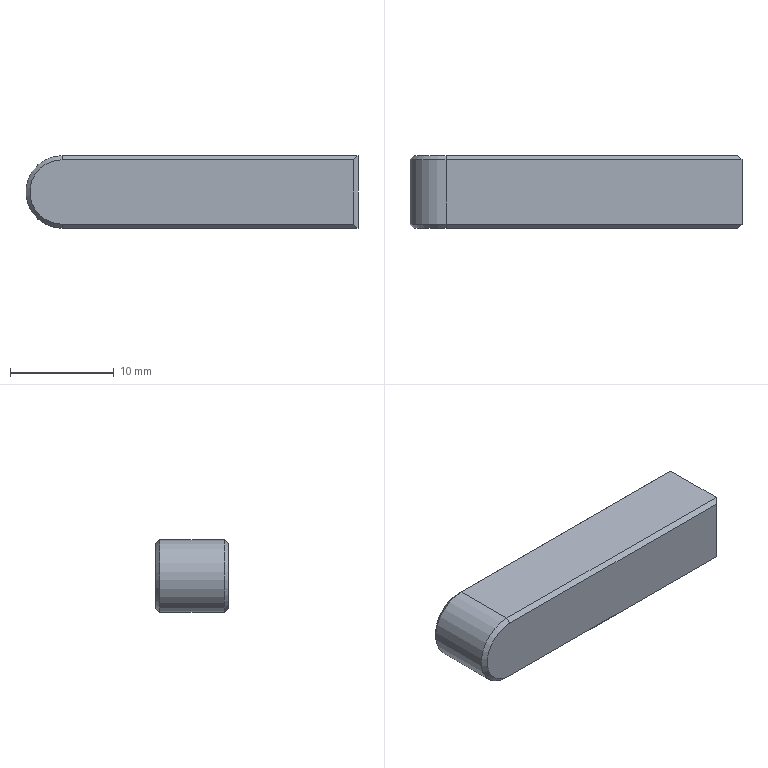Part | SolidWorks | features Chamfer 1, Extrusion 1 | 1 solid | 14 faces | box 32 x 7 x 7 mm | volume 1519 mm3 | plane 11 | cone 2 | cylinder 1 | commonest cylinder face diameters 7 x1
STEP:
#1=CARTESIAN_POINT('',(3.5,6.6,7.));
#2=VERTEX_POINT('',#1);
#3=CARTESIAN_POINT('',(3.5,0.4,7.));
#4=VERTEX_POINT('',#3);
#5=CARTESIAN_POINT('',(3.5,7.,7.));
#6=DIRECTION('',(0.,-1.,0.));
#7=VECTOR('',#6,1000.);
#8=LINE('',#5,#7);
#9=EDGE_CURVE('',#2,#4,#8,.T.);
#10=ORIENTED_EDGE('',*,*,#9,.F.);
#11=CARTESIAN_POINT('',(3.5,6.6,0.));
#12=VERTEX_POINT('',#11);
#13=CARTESIAN_POINT('',(3.5,6.6,3.5));
#14=DIRECTION('',(0.,-1.,0.));
#15=DIRECTION('',(0.,0.,1.));
#16=AXIS2_PLACEMENT_3D('',#13,#14,#15);
#17=CIRCLE('',#16,3.5);
#18=EDGE_CURVE('',#2,#12,#17,.T.);
#19=ORIENTED_EDGE('',*,*,#18,.T.);
#20=CARTESIAN_POINT('',(3.5,0.4,0.));
#21=VERTEX_POINT('',#20);
#22=CARTESIAN_POINT('',(3.5,7.,0.));
#23=DIRECTION('',(0.,-1.,0.));
#24=VECTOR('',#23,1000.);
#25=LINE('',#22,#24);
#26=EDGE_CURVE('',#12,#21,#25,.T.);
#27=ORIENTED_EDGE('',*,*,#26,.T.);
#28=CARTESIAN_POINT('',(3.5,0.4,3.5));
#29=DIRECTION('',(0.,1.,0.));
#30=DIRECTION('',(0.,0.,1.));
#31=AXIS2_PLACEMENT_3D('',#28,#29,#30);
#32=CIRCLE('',#31,3.5);
#33=EDGE_CURVE('',#21,#4,#32,.T.);
#34=ORIENTED_EDGE('',*,*,#33,.T.);
#35=EDGE_LOOP('',(#10,#19,#27,#34));
#36=FACE_OUTER_BOUND('',#35,.T.);
#37=CARTESIAN_POINT('',(3.5,7.,3.5));
#38=DIRECTION('',(0.,-1.,0.));
#39=DIRECTION('',(0.,0.,-1.));
#40=AXIS2_PLACEMENT_3D('',#37,#38,#39);
#41=CYLINDRICAL_SURFACE('',#40,3.5);
#42=ADVANCED_FACE('',(#36),#41,.T.);
#43=CARTESIAN_POINT('',(32.,6.6,7.));
#44=VERTEX_POINT('',#43);
#45=CARTESIAN_POINT('',(32.,0.4,7.));
#46=VERTEX_POINT('',#45);
#47=CARTESIAN_POINT('',(32.,7.,7.));
#48=DIRECTION('',(0.,-1.,0.));
#49=VECTOR('',#48,1000.);
#50=LINE('',#47,#49);
#51=EDGE_CURVE('',#44,#46,#50,.T.);
#52=ORIENTED_EDGE('',*,*,#51,.F.);
#53=CARTESIAN_POINT('',(3.5,6.6,7.));
#54=DIRECTION('',(-1.,0.,0.));
#55=VECTOR('',#54,1000.);
#56=LINE('',#53,#55);
#57=EDGE_CURVE('',#44,#2,#56,.T.);
#58=ORIENTED_EDGE('',*,*,#57,.T.);
#59=ORIENTED_EDGE('',*,*,#9,.T.);
#60=CARTESIAN_POINT('',(3.5,0.4,7.));
#61=DIRECTION('',(1.,0.,0.));
#62=VECTOR('',#61,1000.);
#63=LINE('',#60,#62);
#64=EDGE_CURVE('',#4,#46,#63,.T.);
#65=ORIENTED_EDGE('',*,*,#64,.T.);
#66=EDGE_LOOP('',(#52,#58,#59,#65));
#67=FACE_OUTER_BOUND('',#66,.T.);
#68=CARTESIAN_POINT('',(3.5,7.,7.));
#69=DIRECTION('',(0.,0.,-1.));
#70=DIRECTION('',(-1.,0.,0.));
#71=AXIS2_PLACEMENT_3D('',#68,#69,#70);
#72=PLANE('',#71);
#73=ADVANCED_FACE('',(#67),#72,.F.);
#74=CARTESIAN_POINT('',(32.,6.6,0.));
#75=VERTEX_POINT('',#74);
#76=CARTESIAN_POINT('',(32.,0.4,0.));
#77=VERTEX_POINT('',#76);
#78=CARTESIAN_POINT('',(32.,7.,0.));
#79=DIRECTION('',(0.,-1.,0.));
#80=VECTOR('',#79,1000.);
#81=LINE('',#78,#80);
#82=EDGE_CURVE('',#75,#77,#81,.T.);
#83=ORIENTED_EDGE('',*,*,#82,.F.);
#84=CARTESIAN_POINT('',(32.,6.6,0.));
#85=DIRECTION('',(0.,0.,1.));
#86=VECTOR('',#85,1000.);
#87=LINE('',#84,#86);
#88=EDGE_CURVE('',#75,#44,#87,.T.);
#89=ORIENTED_EDGE('',*,*,#88,.T.);
#90=ORIENTED_EDGE('',*,*,#51,.T.);
#91=CARTESIAN_POINT('',(32.,0.4,0.));
#92=DIRECTION('',(0.,0.,-1.));
#93=VECTOR('',#92,1000.);
#94=LINE('',#91,#93);
#95=EDGE_CURVE('',#46,#77,#94,.T.);
#96=ORIENTED_EDGE('',*,*,#95,.T.);
#97=EDGE_LOOP('',(#83,#89,#90,#96));
#98=FACE_OUTER_BOUND('',#97,.T.);
#99=CARTESIAN_POINT('',(32.,7.,0.));
#100=DIRECTION('',(1.,0.,0.));
#101=DIRECTION('',(0.,0.,-1.));
#102=AXIS2_PLACEMENT_3D('',#99,#100,#101);
#103=PLANE('',#102);
#104=ADVANCED_FACE('',(#98),#103,.T.);
#105=ORIENTED_EDGE('',*,*,#26,.F.);
#106=CARTESIAN_POINT('',(3.5,6.6,0.));
#107=DIRECTION('',(1.,0.,0.));
#108=VECTOR('',#107,1000.);
#109=LINE('',#106,#108);
#110=EDGE_CURVE('',#12,#75,#109,.T.);
#111=ORIENTED_EDGE('',*,*,#110,.T.);
#112=ORIENTED_EDGE('',*,*,#82,.T.);
#113=CARTESIAN_POINT('',(3.5,0.4,0.));
#114=DIRECTION('',(-1.,0.,0.));
#115=VECTOR('',#114,1000.);
#116=LINE('',#113,#115);
#117=EDGE_CURVE('',#77,#21,#116,.T.);
#118=ORIENTED_EDGE('',*,*,#117,.T.);
#119=EDGE_LOOP('',(#105,#111,#112,#118));
#120=FACE_OUTER_BOUND('',#119,.T.);
#121=CARTESIAN_POINT('',(3.5,7.,0.));
#122=DIRECTION('',(0.,0.,-1.));
#123=DIRECTION('',(-1.,0.,0.));
#124=AXIS2_PLACEMENT_3D('',#121,#122,#123);
#125=PLANE('',#124);
#126=ADVANCED_FACE('',(#120),#125,.T.);
#127=CARTESIAN_POINT('',(3.5,7.,6.6));
#128=VERTEX_POINT('',#127);
#129=CARTESIAN_POINT('',(31.6,7.,6.6));
#130=VERTEX_POINT('',#129);
#131=CARTESIAN_POINT('',(32.,7.,6.6));
#132=DIRECTION('',(1.,0.,0.));
#133=VECTOR('',#132,1000.);
#134=LINE('',#131,#133);
#135=EDGE_CURVE('',#128,#130,#134,.T.);
#136=ORIENTED_EDGE('',*,*,#135,.T.);
#137=CARTESIAN_POINT('',(31.6,7.,0.4));
#138=VERTEX_POINT('',#137);
#139=CARTESIAN_POINT('',(31.6,7.,3.5));
#140=DIRECTION('',(0.,0.,-1.));
#141=VECTOR('',#140,1000.);
#142=LINE('',#139,#141);
#143=EDGE_CURVE('',#130,#138,#142,.T.);
#144=ORIENTED_EDGE('',*,*,#143,.T.);
#145=CARTESIAN_POINT('',(3.5,7.,0.4));
#146=VERTEX_POINT('',#145);
#147=CARTESIAN_POINT('',(3.5,7.,0.4));
#148=DIRECTION('',(-1.,0.,0.));
#149=VECTOR('',#148,1000.);
#150=LINE('',#147,#149);
#151=EDGE_CURVE('',#138,#146,#150,.T.);
#152=ORIENTED_EDGE('',*,*,#151,.T.);
#153=CARTESIAN_POINT('',(3.5,7.,3.5));
#154=DIRECTION('',(0.,1.,0.));
#155=DIRECTION('',(0.,0.,1.));
#156=AXIS2_PLACEMENT_3D('',#153,#154,#155);
#157=CIRCLE('',#156,3.1);
#158=EDGE_CURVE('',#146,#128,#157,.T.);
#159=ORIENTED_EDGE('',*,*,#158,.T.);
#160=EDGE_LOOP('',(#136,#144,#152,#159));
#161=FACE_OUTER_BOUND('',#160,.T.);
#162=CARTESIAN_POINT('',(3.5,7.,3.5));
#163=DIRECTION('',(0.,1.,0.));
#164=DIRECTION('',(0.,0.,1.));
#165=AXIS2_PLACEMENT_3D('',#162,#163,#164);
#166=PLANE('',#165);
#167=ADVANCED_FACE('',(#161),#166,.T.);
#168=CARTESIAN_POINT('',(3.5,0.,0.4));
#169=VERTEX_POINT('',#168);
#170=CARTESIAN_POINT('',(31.6,0.,0.4));
#171=VERTEX_POINT('',#170);
#172=CARTESIAN_POINT('',(32.,0.,0.4));
#173=DIRECTION('',(1.,0.,0.));
#174=VECTOR('',#173,1000.);
#175=LINE('',#172,#174);
#176=EDGE_CURVE('',#169,#171,#175,.T.);
#177=ORIENTED_EDGE('',*,*,#176,.T.);
#178=CARTESIAN_POINT('',(31.6,0.,6.6));
#179=VERTEX_POINT('',#178);
#180=CARTESIAN_POINT('',(31.6,0.,7.));
#181=DIRECTION('',(0.,0.,1.));
#182=VECTOR('',#181,1000.);
#183=LINE('',#180,#182);
#184=EDGE_CURVE('',#171,#179,#183,.T.);
#185=ORIENTED_EDGE('',*,*,#184,.T.);
#186=CARTESIAN_POINT('',(3.5,0.,6.6));
#187=VERTEX_POINT('',#186);
#188=CARTESIAN_POINT('',(3.5,0.,6.6));
#189=DIRECTION('',(-1.,0.,0.));
#190=VECTOR('',#189,1000.);
#191=LINE('',#188,#190);
#192=EDGE_CURVE('',#179,#187,#191,.T.);
#193=ORIENTED_EDGE('',*,*,#192,.T.);
#194=CARTESIAN_POINT('',(3.5,0.,3.5));
#195=DIRECTION('',(0.,-1.,0.));
#196=DIRECTION('',(0.,0.,1.));
#197=AXIS2_PLACEMENT_3D('',#194,#195,#196);
#198=CIRCLE('',#197,3.1);
#199=EDGE_CURVE('',#187,#169,#198,.T.);
#200=ORIENTED_EDGE('',*,*,#199,.T.);
#201=EDGE_LOOP('',(#177,#185,#193,#200));
#202=FACE_OUTER_BOUND('',#201,.T.);
#203=CARTESIAN_POINT('',(3.5,0.,3.5));
#204=DIRECTION('',(0.,1.,0.));
#205=DIRECTION('',(0.,0.,1.));
#206=AXIS2_PLACEMENT_3D('',#203,#204,#205);
#207=PLANE('',#206);
#208=ADVANCED_FACE('',(#202),#207,.F.);
#209=CARTESIAN_POINT('',(3.5,7.,6.6));
#210=DIRECTION('',(0.,-0.7071,0.7071));
#211=VECTOR('',#210,1000.);
#212=LINE('',#209,#211);
#213=EDGE_CURVE('',#128,#2,#212,.T.);
#214=ORIENTED_EDGE('',*,*,#213,.F.);
#215=ORIENTED_EDGE('',*,*,#158,.F.);
#216=CARTESIAN_POINT('',(3.5,6.6,0.));
#217=DIRECTION('',(0.,0.7071,0.7071));
#218=VECTOR('',#217,1000.);
#219=LINE('',#216,#218);
#220=EDGE_CURVE('',#12,#146,#219,.T.);
#221=ORIENTED_EDGE('',*,*,#220,.F.);
#222=ORIENTED_EDGE('',*,*,#18,.F.);
#223=EDGE_LOOP('',(#214,#215,#221,#222));
#224=FACE_OUTER_BOUND('',#223,.T.);
#225=CARTESIAN_POINT('',(3.5,7.,3.5));
#226=DIRECTION('',(0.,-1.,0.));
#227=DIRECTION('',(0.,0.,-1.));
#228=AXIS2_PLACEMENT_3D('',#225,#226,#227);
#229=CONICAL_SURFACE('',#228,3.1,0.7854);
#230=ADVANCED_FACE('',(#224),#229,.T.);
#231=ORIENTED_EDGE('',*,*,#220,.T.);
#232=ORIENTED_EDGE('',*,*,#151,.F.);
#233=CARTESIAN_POINT('',(22.5,16.1,9.5));
#234=DIRECTION('',(-0.5774,0.5774,0.5774));
#235=VECTOR('',#234,1000.);
#236=LINE('',#233,#235);
#237=EDGE_CURVE('',#75,#138,#236,.T.);
#238=ORIENTED_EDGE('',*,*,#237,.F.);
#239=ORIENTED_EDGE('',*,*,#110,.F.);
#240=EDGE_LOOP('',(#231,#232,#238,#239));
#241=FACE_OUTER_BOUND('',#240,.T.);
#242=CARTESIAN_POINT('',(3.5,6.6,0.));
#243=DIRECTION('',(0.,-0.7071,0.7071));
#244=DIRECTION('',(1.,0.,0.));
#245=AXIS2_PLACEMENT_3D('',#242,#243,#244);
#246=PLANE('',#245);
#247=ADVANCED_FACE('',(#241),#246,.F.);
#248=ORIENTED_EDGE('',*,*,#213,.T.);
#249=ORIENTED_EDGE('',*,*,#57,.F.);
#250=CARTESIAN_POINT('',(22.233,16.367,-2.767));
#251=DIRECTION('',(0.5774,-0.5774,0.5774));
#252=VECTOR('',#251,1000.);
#253=LINE('',#250,#252);
#254=EDGE_CURVE('',#130,#44,#253,.T.);
#255=ORIENTED_EDGE('',*,*,#254,.F.);
#256=ORIENTED_EDGE('',*,*,#135,.F.);
#257=EDGE_LOOP('',(#248,#249,#255,#256));
#258=FACE_OUTER_BOUND('',#257,.T.);
#259=CARTESIAN_POINT('',(3.5,7.,6.6));
#260=DIRECTION('',(0.,0.7071,0.7071));
#261=DIRECTION('',(-1.,0.,0.));
#262=AXIS2_PLACEMENT_3D('',#259,#260,#261);
#263=PLANE('',#262);
#264=ADVANCED_FACE('',(#258),#263,.T.);
#265=ORIENTED_EDGE('',*,*,#237,.T.);
#266=ORIENTED_EDGE('',*,*,#143,.F.);
#267=ORIENTED_EDGE('',*,*,#254,.T.);
#268=ORIENTED_EDGE('',*,*,#88,.F.);
#269=EDGE_LOOP('',(#265,#266,#267,#268));
#270=FACE_OUTER_BOUND('',#269,.T.);
#271=CARTESIAN_POINT('',(32.,6.6,0.));
#272=DIRECTION('',(-0.7071,-0.7071,0.));
#273=DIRECTION('',(0.,0.,1.));
#274=AXIS2_PLACEMENT_3D('',#271,#272,#273);
#275=PLANE('',#274);
#276=ADVANCED_FACE('',(#270),#275,.F.);
#277=CARTESIAN_POINT('',(3.5,0.4,7.));
#278=DIRECTION('',(0.,-0.7071,-0.7071));
#279=VECTOR('',#278,1000.);
#280=LINE('',#277,#279);
#281=EDGE_CURVE('',#4,#187,#280,.T.);
#282=ORIENTED_EDGE('',*,*,#281,.F.);
#283=ORIENTED_EDGE('',*,*,#33,.F.);
#284=CARTESIAN_POINT('',(3.5,0.,0.4));
#285=DIRECTION('',(0.,0.7071,-0.7071));
#286=VECTOR('',#285,1000.);
#287=LINE('',#284,#286);
#288=EDGE_CURVE('',#169,#21,#287,.T.);
#289=ORIENTED_EDGE('',*,*,#288,.F.);
#290=ORIENTED_EDGE('',*,*,#199,.F.);
#291=EDGE_LOOP('',(#282,#283,#289,#290));
#292=FACE_OUTER_BOUND('',#291,.T.);
#293=CARTESIAN_POINT('',(3.5,0.4,3.5));
#294=DIRECTION('',(0.,1.,0.));
#295=DIRECTION('',(0.,0.,1.));
#296=AXIS2_PLACEMENT_3D('',#293,#294,#295);
#297=CONICAL_SURFACE('',#296,3.5,0.7854);
#298=ADVANCED_FACE('',(#292),#297,.T.);
#299=ORIENTED_EDGE('',*,*,#288,.T.);
#300=ORIENTED_EDGE('',*,*,#117,.F.);
#301=CARTESIAN_POINT('',(22.233,-9.367,9.767));
#302=DIRECTION('',(0.5774,0.5774,-0.5774));
#303=VECTOR('',#302,1000.);
#304=LINE('',#301,#303);
#305=EDGE_CURVE('',#171,#77,#304,.T.);
#306=ORIENTED_EDGE('',*,*,#305,.F.);
#307=ORIENTED_EDGE('',*,*,#176,.F.);
#308=EDGE_LOOP('',(#299,#300,#306,#307));
#309=FACE_OUTER_BOUND('',#308,.T.);
#310=CARTESIAN_POINT('',(3.5,0.,0.4));
#311=DIRECTION('',(0.,-0.7071,-0.7071));
#312=DIRECTION('',(-1.,0.,0.));
#313=AXIS2_PLACEMENT_3D('',#310,#311,#312);
#314=PLANE('',#313);
#315=ADVANCED_FACE('',(#309),#314,.T.);
#316=ORIENTED_EDGE('',*,*,#281,.T.);
#317=ORIENTED_EDGE('',*,*,#192,.F.);
#318=CARTESIAN_POINT('',(22.5,-9.1,-2.5));
#319=DIRECTION('',(-0.5774,-0.5774,-0.5774));
#320=VECTOR('',#319,1000.);
#321=LINE('',#318,#320);
#322=EDGE_CURVE('',#46,#179,#321,.T.);
#323=ORIENTED_EDGE('',*,*,#322,.F.);
#324=ORIENTED_EDGE('',*,*,#64,.F.);
#325=EDGE_LOOP('',(#316,#317,#323,#324));
#326=FACE_OUTER_BOUND('',#325,.T.);
#327=CARTESIAN_POINT('',(3.5,0.4,7.));
#328=DIRECTION('',(0.,0.7071,-0.7071));
#329=DIRECTION('',(1.,0.,0.));
#330=AXIS2_PLACEMENT_3D('',#327,#328,#329);
#331=PLANE('',#330);
#332=ADVANCED_FACE('',(#326),#331,.F.);
#333=ORIENTED_EDGE('',*,*,#305,.T.);
#334=ORIENTED_EDGE('',*,*,#95,.F.);
#335=ORIENTED_EDGE('',*,*,#322,.T.);
#336=ORIENTED_EDGE('',*,*,#184,.F.);
#337=EDGE_LOOP('',(#333,#334,#335,#336));
#338=FACE_OUTER_BOUND('',#337,.T.);
#339=CARTESIAN_POINT('',(31.6,0.,3.5));
#340=DIRECTION('',(0.7071,-0.7071,0.));
#341=DIRECTION('',(0.,0.,-1.));
#342=AXIS2_PLACEMENT_3D('',#339,#340,#341);
#343=PLANE('',#342);
#344=ADVANCED_FACE('',(#338),#343,.T.);
#345=CLOSED_SHELL('',(#42,#73,#104,#126,#167,#208,#230,#247,#264,#276,#298,#315,#332,#344));
#346=MANIFOLD_SOLID_BREP('',#345);
#347=CARTESIAN_POINT('',(0.,0.,0.));
#348=DIRECTION('',(0.,0.,1.));
#349=DIRECTION('',(1.,0.,0.));
#350=AXIS2_PLACEMENT_3D('',#347,#348,#349);
#351=(LENGTH_UNIT()NAMED_UNIT(*)SI_UNIT(.MILLI.,.METRE.));
#352=UNCERTAINTY_MEASURE_WITH_UNIT(LENGTH_MEASURE(0.00001),#351,'','');
#353=(NAMED_UNIT(*)PLANE_ANGLE_UNIT()SI_UNIT($,.RADIAN.));
#354=(NAMED_UNIT(*)SI_UNIT($,.STERADIAN.)SOLID_ANGLE_UNIT());
#355=(GEOMETRIC_REPRESENTATION_CONTEXT(3)GLOBAL_UNCERTAINTY_ASSIGNED_CONTEXT((#352))GLOBAL_UNIT_ASSIGNED_CONTEXT((#351,#353,#354))REPRESENTATION_CONTEXT('',''));
#356=ADVANCED_BREP_SHAPE_REPRESENTATION('',(#346,#350),#355);